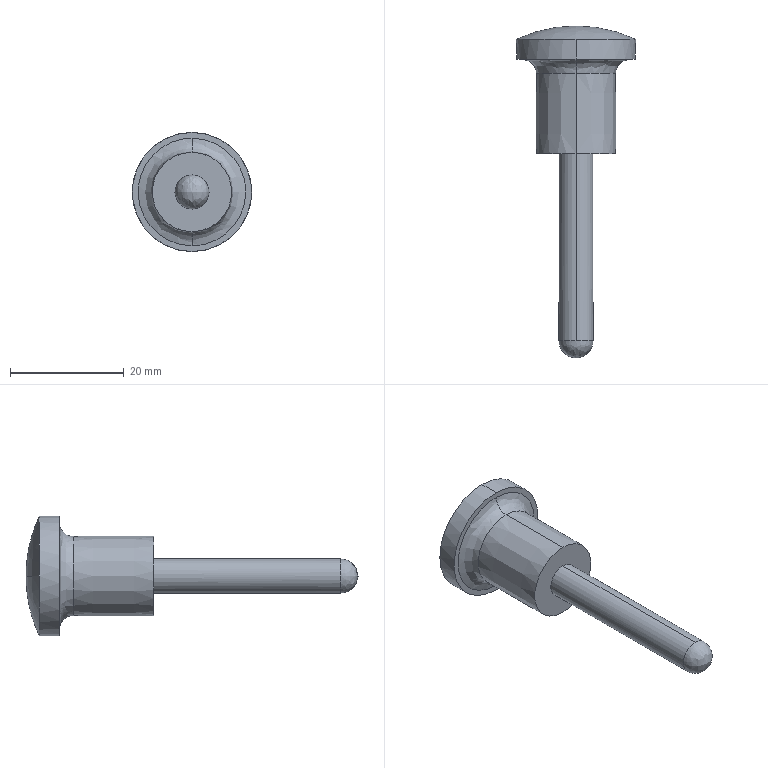Part | SolidWorks | features BaseBody 1 | 1 solid | 13 faces | box 21 x 58.38 x 21 mm | volume 5233 mm3 | spline 5 | cylinder 4 | cone 2 | plane 2 | commonest cylinder face diameters 6 x2 21 x2
STEP:
#1=CARTESIAN_POINT('',(0.,46.16,10.5));
#2=VERTEX_POINT('',#1);
#3=CARTESIAN_POINT('',(10.5,46.16,0.));
#4=VERTEX_POINT('',#3);
#5=CARTESIAN_POINT('',(0.,46.16,0.));
#6=DIRECTION('',(0.,1.,0.));
#7=DIRECTION('',(0.,0.,-1.));
#8=AXIS2_PLACEMENT_3D('',#5,#6,#7);
#9=CIRCLE('',#8,10.5);
#10=EDGE_CURVE('',#2,#4,#9,.T.);
#11=ORIENTED_EDGE('',*,*,#10,.T.);
#12=CARTESIAN_POINT('',(-10.5,46.16,0.));
#13=VERTEX_POINT('',#12);
#14=CARTESIAN_POINT('',(0.,23.772,0.));
#15=DIRECTION('',(0.,0.,1.));
#16=DIRECTION('',(1.,0.,0.));
#17=AXIS2_PLACEMENT_3D('',#14,#15,#16);
#18=CIRCLE('',#17,24.728);
#19=EDGE_CURVE('',#4,#13,#18,.T.);
#20=ORIENTED_EDGE('',*,*,#19,.T.);
#21=CARTESIAN_POINT('',(0.,46.16,0.));
#22=DIRECTION('',(0.,1.,0.));
#23=DIRECTION('',(0.,0.,-1.));
#24=AXIS2_PLACEMENT_3D('',#21,#22,#23);
#25=CIRCLE('',#24,10.5);
#26=EDGE_CURVE('',#13,#2,#25,.T.);
#27=ORIENTED_EDGE('',*,*,#26,.T.);
#28=EDGE_LOOP('',(#11,#20,#27));
#29=FACE_OUTER_BOUND('',#28,.T.);
#30=CARTESIAN_POINT('',(10.618,46.104,0.));
#31=CARTESIAN_POINT('',(10.618,46.104,3.311));
#32=CARTESIAN_POINT('',(10.618,45.38,6.542));
#33=CARTESIAN_POINT('',(10.618,43.966,9.536));
#34=CARTESIAN_POINT('',(3.784,49.354,0.));
#35=CARTESIAN_POINT('',(3.784,49.354,3.793));
#36=CARTESIAN_POINT('',(3.784,48.524,7.494));
#37=CARTESIAN_POINT('',(3.784,46.904,10.923));
#38=CARTESIAN_POINT('',(-3.784,49.354,0.));
#39=CARTESIAN_POINT('',(-3.784,49.354,3.793));
#40=CARTESIAN_POINT('',(-3.784,48.524,7.494));
#41=CARTESIAN_POINT('',(-3.784,46.904,10.923));
#42=CARTESIAN_POINT('',(-10.618,46.104,0.));
#43=CARTESIAN_POINT('',(-10.618,46.104,3.311));
#44=CARTESIAN_POINT('',(-10.618,45.38,6.542));
#45=CARTESIAN_POINT('',(-10.618,43.966,9.536));
#46=(BOUNDED_SURFACE()B_SPLINE_SURFACE(3,3,((#30,#31,#32,#33),(#34,#35,#36,#37),(#38,#39,#40,#41),(#42,#43,#44,#45)),.UNSPECIFIED.,.F.,.F.,.F.)B_SPLINE_SURFACE_WITH_KNOTS((4,4),(4,4),(0.,1.),(0.,1.),.UNSPECIFIED.)GEOMETRIC_REPRESENTATION_ITEM()RATIONAL_B_SPLINE_SURFACE(((1.,0.9838,0.9838,1.),(0.9354,0.9203,0.9203,0.9354),(0.9354,0.9203,0.9203,0.9354),(1.,0.9838,0.9838,1.)))REPRESENTATION_ITEM('')SURFACE());
#47=ADVANCED_FACE('',(#29),#46,.T.);
#48=CARTESIAN_POINT('',(0.,40.146,-6.975));
#49=VERTEX_POINT('',#48);
#50=CARTESIAN_POINT('',(0.,40.146,6.975));
#51=VERTEX_POINT('',#50);
#52=CARTESIAN_POINT('',(0.,40.146,0.));
#53=DIRECTION('',(0.,-1.,0.));
#54=DIRECTION('',(0.,0.,1.));
#55=AXIS2_PLACEMENT_3D('',#52,#53,#54);
#56=CIRCLE('',#55,6.975);
#57=EDGE_CURVE('',#49,#51,#56,.T.);
#58=ORIENTED_EDGE('',*,*,#57,.F.);
#59=CARTESIAN_POINT('',(0.,42.65,-9.475));
#60=VERTEX_POINT('',#59);
#61=CARTESIAN_POINT('',(0.,40.15,-9.475));
#62=DIRECTION('',(-1.,0.,0.));
#63=DIRECTION('',(0.,0.,-1.));
#64=AXIS2_PLACEMENT_3D('',#61,#62,#63);
#65=CIRCLE('',#64,2.5);
#66=EDGE_CURVE('',#49,#60,#65,.T.);
#67=ORIENTED_EDGE('',*,*,#66,.T.);
#68=CARTESIAN_POINT('',(9.475,42.65,0.));
#69=VERTEX_POINT('',#68);
#70=CARTESIAN_POINT('',(9.475,42.65,0.));
#71=CARTESIAN_POINT('',(9.475,42.65,-0.2897));
#72=CARTESIAN_POINT('',(9.456,42.65,-0.7225));
#73=CARTESIAN_POINT('',(9.398,42.65,-1.224));
#74=CARTESIAN_POINT('',(9.36,42.65,-1.475));
#75=CARTESIAN_POINT('',(9.342,42.65,-1.582));
#76=CARTESIAN_POINT('',(9.33,42.65,-1.653));
#77=CARTESIAN_POINT('',(9.324,42.65,-1.686));
#78=CARTESIAN_POINT('',(9.261,42.65,-2.026));
#79=CARTESIAN_POINT('',(9.156,42.65,-2.473));
#80=CARTESIAN_POINT('',(8.996,42.65,-2.984));
#81=CARTESIAN_POINT('',(8.906,42.65,-3.237));
#82=CARTESIAN_POINT('',(8.865,42.65,-3.345));
#83=CARTESIAN_POINT('',(8.838,42.65,-3.416));
#84=CARTESIAN_POINT('',(8.825,42.65,-3.451));
#85=CARTESIAN_POINT('',(8.692,42.65,-3.785));
#86=CARTESIAN_POINT('',(8.494,42.65,-4.221));
#87=CARTESIAN_POINT('',(8.225,42.65,-4.709));
#88=CARTESIAN_POINT('',(8.102,42.65,-4.915));
#89=CARTESIAN_POINT('',(8.018,42.65,-5.05));
#90=CARTESIAN_POINT('',(7.976,42.65,-5.117));
#91=CARTESIAN_POINT('',(7.573,42.65,-5.732));
#92=CARTESIAN_POINT('',(7.162,42.65,-6.238));
#93=CARTESIAN_POINT('',(6.469,42.65,-6.931));
#94=CARTESIAN_POINT('',(6.106,42.65,-7.258));
#95=CARTESIAN_POINT('',(5.655,42.65,-7.606));
#96=CARTESIAN_POINT('',(5.456,42.65,-7.748));
#97=CARTESIAN_POINT('',(5.321,42.65,-7.84));
#98=CARTESIAN_POINT('',(5.252,42.65,-7.887));
#99=CARTESIAN_POINT('',(4.917,42.65,-8.106));
#100=CARTESIAN_POINT('',(4.504,42.65,-8.347));
#101=CARTESIAN_POINT('',(4.003,42.65,-8.591));
#102=CARTESIAN_POINT('',(3.747,42.65,-8.704));
#103=CARTESIAN_POINT('',(3.636,42.65,-8.75));
#104=CARTESIAN_POINT('',(3.562,42.65,-8.78));
#105=CARTESIAN_POINT('',(3.524,42.65,-8.796));
#106=CARTESIAN_POINT('',(3.202,42.65,-8.923));
#107=CARTESIAN_POINT('',(2.768,42.65,-9.071));
#108=CARTESIAN_POINT('',(2.25,42.65,-9.207));
#109=CARTESIAN_POINT('',(1.988,42.65,-9.265));
#110=CARTESIAN_POINT('',(1.875,42.65,-9.288));
#111=CARTESIAN_POINT('',(1.8,42.65,-9.303));
#112=CARTESIAN_POINT('',(1.76,42.65,-9.311));
#113=CARTESIAN_POINT('',(1.154,42.65,-9.423));
#114=CARTESIAN_POINT('',(0.5797,42.65,-9.475));
#115=CARTESIAN_POINT('',(0.,42.65,-9.475));
#116=B_SPLINE_CURVE_WITH_KNOTS('',3,(#70,#71,#72,#73,#74,#75,#76,#77,#78,#79,#80,#81,#82,#83,#84,#85,#86,#87,#88,#89,#90,#91,#92,#93,#94,#95,#96,#97,#98,#99,#100,#101,#102,#103,#104,#105,#106,#107,#108,#109,#110,#111,#112,#113,#114,#115),.UNSPECIFIED.,.F.,.F.,(4,1,1,1,2,2,1,1,1,2,2,1,1,2,2,2,1,1,2,2,1,1,1,2,2,1,1,1,2,2,4),(0.,0.0625,0.09375,0.1094,0.1172,0.125,0.1875,0.2187,0.2344,0.2422,0.25,0.3125,0.3437,0.3594,0.375,0.5,0.5625,0.5938,0.6094,0.625,0.6875,0.7188,0.7344,0.7422,0.75,0.8125,0.8438,0.8594,0.8672,0.875,1.),.UNSPECIFIED.);
#117=EDGE_CURVE('',#69,#60,#116,.T.);
#118=ORIENTED_EDGE('',*,*,#117,.F.);
#119=CARTESIAN_POINT('',(0.,42.65,9.475));
#120=VERTEX_POINT('',#119);
#121=CARTESIAN_POINT('',(0.,42.65,9.475));
#122=CARTESIAN_POINT('',(0.2897,42.65,9.475));
#123=CARTESIAN_POINT('',(0.7225,42.65,9.456));
#124=CARTESIAN_POINT('',(1.224,42.65,9.398));
#125=CARTESIAN_POINT('',(1.475,42.65,9.36));
#126=CARTESIAN_POINT('',(1.582,42.65,9.342));
#127=CARTESIAN_POINT('',(1.653,42.65,9.33));
#128=CARTESIAN_POINT('',(1.686,42.65,9.324));
#129=CARTESIAN_POINT('',(2.026,42.65,9.261));
#130=CARTESIAN_POINT('',(2.473,42.65,9.156));
#131=CARTESIAN_POINT('',(2.984,42.65,8.996));
#132=CARTESIAN_POINT('',(3.237,42.65,8.906));
#133=CARTESIAN_POINT('',(3.345,42.65,8.865));
#134=CARTESIAN_POINT('',(3.416,42.65,8.838));
#135=CARTESIAN_POINT('',(3.451,42.65,8.825));
#136=CARTESIAN_POINT('',(3.785,42.65,8.692));
#137=CARTESIAN_POINT('',(4.221,42.65,8.494));
#138=CARTESIAN_POINT('',(4.709,42.65,8.225));
#139=CARTESIAN_POINT('',(4.915,42.65,8.102));
#140=CARTESIAN_POINT('',(5.05,42.65,8.018));
#141=CARTESIAN_POINT('',(5.117,42.65,7.976));
#142=CARTESIAN_POINT('',(5.732,42.65,7.573));
#143=CARTESIAN_POINT('',(6.238,42.65,7.162));
#144=CARTESIAN_POINT('',(6.931,42.65,6.469));
#145=CARTESIAN_POINT('',(7.258,42.65,6.106));
#146=CARTESIAN_POINT('',(7.606,42.65,5.655));
#147=CARTESIAN_POINT('',(7.748,42.65,5.456));
#148=CARTESIAN_POINT('',(7.84,42.65,5.321));
#149=CARTESIAN_POINT('',(7.887,42.65,5.252));
#150=CARTESIAN_POINT('',(8.106,42.65,4.917));
#151=CARTESIAN_POINT('',(8.347,42.65,4.504));
#152=CARTESIAN_POINT('',(8.591,42.65,4.003));
#153=CARTESIAN_POINT('',(8.704,42.65,3.747));
#154=CARTESIAN_POINT('',(8.75,42.65,3.636));
#155=CARTESIAN_POINT('',(8.78,42.65,3.562));
#156=CARTESIAN_POINT('',(8.796,42.65,3.524));
#157=CARTESIAN_POINT('',(8.923,42.65,3.202));
#158=CARTESIAN_POINT('',(9.071,42.65,2.768));
#159=CARTESIAN_POINT('',(9.207,42.65,2.25));
#160=CARTESIAN_POINT('',(9.265,42.65,1.988));
#161=CARTESIAN_POINT('',(9.288,42.65,1.875));
#162=CARTESIAN_POINT('',(9.303,42.65,1.8));
#163=CARTESIAN_POINT('',(9.311,42.65,1.76));
#164=CARTESIAN_POINT('',(9.423,42.65,1.154));
#165=CARTESIAN_POINT('',(9.475,42.65,0.5797));
#166=CARTESIAN_POINT('',(9.475,42.65,0.));
#167=B_SPLINE_CURVE_WITH_KNOTS('',3,(#121,#122,#123,#124,#125,#126,#127,#128,#129,#130,#131,#132,#133,#134,#135,#136,#137,#138,#139,#140,#141,#142,#143,#144,#145,#146,#147,#148,#149,#150,#151,#152,#153,#154,#155,#156,#157,#158,#159,#160,#161,#162,#163,#164,#165,#166),.UNSPECIFIED.,.F.,.F.,(4,1,1,1,2,2,1,1,1,2,2,1,1,2,2,2,1,1,2,2,1,1,1,2,2,1,1,1,2,2,4),(0.,0.0625,0.09375,0.1094,0.1172,0.125,0.1875,0.2188,0.2344,0.2422,0.25,0.3125,0.3438,0.3594,0.375,0.5,0.5625,0.5938,0.6094,0.625,0.6875,0.7188,0.7344,0.7422,0.75,0.8125,0.8438,0.8594,0.8672,0.875,1.),.UNSPECIFIED.);
#168=EDGE_CURVE('',#120,#69,#167,.T.);
#169=ORIENTED_EDGE('',*,*,#168,.F.);
#170=CARTESIAN_POINT('',(0.,40.15,9.475));
#171=DIRECTION('',(1.,0.,0.));
#172=DIRECTION('',(0.,0.,1.));
#173=AXIS2_PLACEMENT_3D('',#170,#171,#172);
#174=CIRCLE('',#173,2.5);
#175=EDGE_CURVE('',#51,#120,#174,.T.);
#176=ORIENTED_EDGE('',*,*,#175,.F.);
#177=EDGE_LOOP('',(#58,#67,#118,#169,#176));
#178=FACE_OUTER_BOUND('',#177,.T.);
#179=CARTESIAN_POINT('',(0.,40.146,6.975));
#180=CARTESIAN_POINT('',(13.951,40.146,6.975));
#181=CARTESIAN_POINT('',(13.951,40.146,-6.975));
#182=CARTESIAN_POINT('',(0.,40.146,-6.975));
#183=CARTESIAN_POINT('',(0.,41.612,6.973));
#184=CARTESIAN_POINT('',(13.946,41.612,6.973));
#185=CARTESIAN_POINT('',(13.946,41.612,-6.973));
#186=CARTESIAN_POINT('',(0.,41.612,-6.973));
#187=CARTESIAN_POINT('',(0.,42.65,8.009));
#188=CARTESIAN_POINT('',(16.018,42.65,8.009));
#189=CARTESIAN_POINT('',(16.018,42.65,-8.009));
#190=CARTESIAN_POINT('',(0.,42.65,-8.009));
#191=CARTESIAN_POINT('',(0.,42.65,9.475));
#192=CARTESIAN_POINT('',(18.951,42.65,9.475));
#193=CARTESIAN_POINT('',(18.951,42.65,-9.475));
#194=CARTESIAN_POINT('',(0.,42.65,-9.475));
#195=(BOUNDED_SURFACE()B_SPLINE_SURFACE(3,3,((#179,#180,#181,#182),(#183,#184,#185,#186),(#187,#188,#189,#190),(#191,#192,#193,#194)),.UNSPECIFIED.,.F.,.F.,.F.)B_SPLINE_SURFACE_WITH_KNOTS((4,4),(4,4),(0.,1.),(0.,1.),.UNSPECIFIED.)GEOMETRIC_REPRESENTATION_ITEM()RATIONAL_B_SPLINE_SURFACE(((1.,0.3333,0.3333,1.),(0.8043,0.2681,0.2681,0.8043),(0.8043,0.2681,0.2681,0.8043),(1.,0.3333,0.3333,1.)))REPRESENTATION_ITEM('')SURFACE());
#196=ADVANCED_FACE('',(#178),#195,.F.);
#197=ORIENTED_EDGE('',*,*,#10,.F.);
#198=CARTESIAN_POINT('',(0.,42.65,10.5));
#199=VERTEX_POINT('',#198);
#200=CARTESIAN_POINT('',(0.,44.405,10.5));
#201=DIRECTION('',(0.,-1.,0.));
#202=VECTOR('',#201,1000.);
#203=LINE('',#200,#202);
#204=EDGE_CURVE('',#2,#199,#203,.T.);
#205=ORIENTED_EDGE('',*,*,#204,.T.);
#206=CARTESIAN_POINT('',(0.,42.65,-10.5));
#207=VERTEX_POINT('',#206);
#208=CARTESIAN_POINT('',(0.,42.65,0.));
#209=DIRECTION('',(0.,1.,0.));
#210=DIRECTION('',(0.,0.,-1.));
#211=AXIS2_PLACEMENT_3D('',#208,#209,#210);
#212=CIRCLE('',#211,10.5);
#213=EDGE_CURVE('',#199,#207,#212,.T.);
#214=ORIENTED_EDGE('',*,*,#213,.T.);
#215=CARTESIAN_POINT('',(0.,46.16,-10.5));
#216=VERTEX_POINT('',#215);
#217=CARTESIAN_POINT('',(0.,44.405,-10.5));
#218=DIRECTION('',(0.,-1.,0.));
#219=VECTOR('',#218,1000.);
#220=LINE('',#217,#219);
#221=EDGE_CURVE('',#216,#207,#220,.T.);
#222=ORIENTED_EDGE('',*,*,#221,.F.);
#223=CARTESIAN_POINT('',(0.,46.16,0.));
#224=DIRECTION('',(0.,1.,0.));
#225=DIRECTION('',(0.,0.,-1.));
#226=AXIS2_PLACEMENT_3D('',#223,#224,#225);
#227=CIRCLE('',#226,10.5);
#228=EDGE_CURVE('',#4,#216,#227,.T.);
#229=ORIENTED_EDGE('',*,*,#228,.F.);
#230=EDGE_LOOP('',(#197,#205,#214,#222,#229));
#231=FACE_OUTER_BOUND('',#230,.T.);
#232=CARTESIAN_POINT('',(0.,44.405,0.));
#233=DIRECTION('',(0.,-1.,0.));
#234=DIRECTION('',(0.,0.,-1.));
#235=AXIS2_PLACEMENT_3D('',#232,#233,#234);
#236=CYLINDRICAL_SURFACE('',#235,10.5);
#237=ADVANCED_FACE('',(#231),#236,.T.);
#238=ORIENTED_EDGE('',*,*,#57,.T.);
#239=CARTESIAN_POINT('',(0.,26.,7.));
#240=VERTEX_POINT('',#239);
#241=CARTESIAN_POINT('',(0.,26.,7.));
#242=DIRECTION('',(0.,-1.,0.001745));
#243=VECTOR('',#242,1000.);
#244=LINE('',#241,#243);
#245=EDGE_CURVE('',#51,#240,#244,.T.);
#246=ORIENTED_EDGE('',*,*,#245,.T.);
#247=CARTESIAN_POINT('',(0.,26.,-7.));
#248=VERTEX_POINT('',#247);
#249=CARTESIAN_POINT('',(0.,26.,0.));
#250=DIRECTION('',(0.,1.,0.));
#251=DIRECTION('',(0.,0.,-1.));
#252=AXIS2_PLACEMENT_3D('',#249,#250,#251);
#253=CIRCLE('',#252,7.);
#254=EDGE_CURVE('',#240,#248,#253,.T.);
#255=ORIENTED_EDGE('',*,*,#254,.T.);
#256=CARTESIAN_POINT('',(0.,26.,-7.));
#257=DIRECTION('',(0.,-1.,-0.001745));
#258=VECTOR('',#257,1000.);
#259=LINE('',#256,#258);
#260=EDGE_CURVE('',#49,#248,#259,.T.);
#261=ORIENTED_EDGE('',*,*,#260,.F.);
#262=EDGE_LOOP('',(#238,#246,#255,#261));
#263=FACE_OUTER_BOUND('',#262,.T.);
#264=CARTESIAN_POINT('',(0.,26.,0.));
#265=DIRECTION('',(0.,-1.,0.));
#266=DIRECTION('',(0.,0.,-1.));
#267=AXIS2_PLACEMENT_3D('',#264,#265,#266);
#268=CONICAL_SURFACE('',#267,7.,0.001745);
#269=ADVANCED_FACE('',(#263),#268,.T.);
#270=CARTESIAN_POINT('',(0.,26.,3.));
#271=VERTEX_POINT('',#270);
#272=CARTESIAN_POINT('',(0.,26.,-3.));
#273=VERTEX_POINT('',#272);
#274=CARTESIAN_POINT('',(0.,26.,0.));
#275=DIRECTION('',(0.,1.,0.));
#276=DIRECTION('',(0.,0.,-1.));
#277=AXIS2_PLACEMENT_3D('',#274,#275,#276);
#278=CIRCLE('',#277,3.);
#279=EDGE_CURVE('',#271,#273,#278,.T.);
#280=ORIENTED_EDGE('',*,*,#279,.F.);
#281=CARTESIAN_POINT('',(0.,-7.,3.));
#282=VERTEX_POINT('',#281);
#283=CARTESIAN_POINT('',(0.,8.05,3.));
#284=DIRECTION('',(0.,-1.,0.));
#285=VECTOR('',#284,1000.);
#286=LINE('',#283,#285);
#287=EDGE_CURVE('',#271,#282,#286,.T.);
#288=ORIENTED_EDGE('',*,*,#287,.T.);
#289=CARTESIAN_POINT('',(3.,-7.,0.));
#290=VERTEX_POINT('',#289);
#291=CARTESIAN_POINT('',(0.,-7.,0.));
#292=DIRECTION('',(0.,1.,0.));
#293=DIRECTION('',(0.,0.,-1.));
#294=AXIS2_PLACEMENT_3D('',#291,#292,#293);
#295=CIRCLE('',#294,3.);
#296=EDGE_CURVE('',#282,#290,#295,.T.);
#297=ORIENTED_EDGE('',*,*,#296,.T.);
#298=CARTESIAN_POINT('',(0.,-7.,-3.));
#299=VERTEX_POINT('',#298);
#300=CARTESIAN_POINT('',(0.,-7.,0.));
#301=DIRECTION('',(0.,1.,0.));
#302=DIRECTION('',(0.,0.,-1.));
#303=AXIS2_PLACEMENT_3D('',#300,#301,#302);
#304=CIRCLE('',#303,3.);
#305=EDGE_CURVE('',#290,#299,#304,.T.);
#306=ORIENTED_EDGE('',*,*,#305,.T.);
#307=CARTESIAN_POINT('',(0.,8.05,-3.));
#308=DIRECTION('',(0.,-1.,0.));
#309=VECTOR('',#308,1000.);
#310=LINE('',#307,#309);
#311=EDGE_CURVE('',#273,#299,#310,.T.);
#312=ORIENTED_EDGE('',*,*,#311,.F.);
#313=EDGE_LOOP('',(#280,#288,#297,#306,#312));
#314=FACE_OUTER_BOUND('',#313,.T.);
#315=CARTESIAN_POINT('',(0.,8.05,0.));
#316=DIRECTION('',(0.,-1.,0.));
#317=DIRECTION('',(0.,0.,-1.));
#318=AXIS2_PLACEMENT_3D('',#315,#316,#317);
#319=CYLINDRICAL_SURFACE('',#318,3.);
#320=ADVANCED_FACE('',(#314),#319,.T.);
#321=ORIENTED_EDGE('',*,*,#19,.F.);
#322=ORIENTED_EDGE('',*,*,#228,.T.);
#323=CARTESIAN_POINT('',(0.,46.16,0.));
#324=DIRECTION('',(0.,1.,0.));
#325=DIRECTION('',(0.,0.,-1.));
#326=AXIS2_PLACEMENT_3D('',#323,#324,#325);
#327=CIRCLE('',#326,10.5);
#328=EDGE_CURVE('',#216,#13,#327,.T.);
#329=ORIENTED_EDGE('',*,*,#328,.T.);
#330=EDGE_LOOP('',(#321,#322,#329));
#331=FACE_OUTER_BOUND('',#330,.T.);
#332=CARTESIAN_POINT('',(10.618,43.966,-9.536));
#333=CARTESIAN_POINT('',(10.618,45.38,-6.542));
#334=CARTESIAN_POINT('',(10.618,46.104,-3.311));
#335=CARTESIAN_POINT('',(10.618,46.104,0.));
#336=CARTESIAN_POINT('',(3.784,46.904,-10.923));
#337=CARTESIAN_POINT('',(3.784,48.524,-7.494));
#338=CARTESIAN_POINT('',(3.784,49.354,-3.793));
#339=CARTESIAN_POINT('',(3.784,49.354,0.));
#340=CARTESIAN_POINT('',(-3.784,46.904,-10.923));
#341=CARTESIAN_POINT('',(-3.784,48.524,-7.494));
#342=CARTESIAN_POINT('',(-3.784,49.354,-3.793));
#343=CARTESIAN_POINT('',(-3.784,49.354,0.));
#344=CARTESIAN_POINT('',(-10.618,43.966,-9.536));
#345=CARTESIAN_POINT('',(-10.618,45.38,-6.542));
#346=CARTESIAN_POINT('',(-10.618,46.104,-3.311));
#347=CARTESIAN_POINT('',(-10.618,46.104,0.));
#348=(BOUNDED_SURFACE()B_SPLINE_SURFACE(3,3,((#332,#333,#334,#335),(#336,#337,#338,#339),(#340,#341,#342,#343),(#344,#345,#346,#347)),.UNSPECIFIED.,.F.,.F.,.F.)B_SPLINE_SURFACE_WITH_KNOTS((4,4),(4,4),(0.,1.),(0.,1.),.UNSPECIFIED.)GEOMETRIC_REPRESENTATION_ITEM()RATIONAL_B_SPLINE_SURFACE(((1.,0.9838,0.9838,1.),(0.9354,0.9203,0.9203,0.9354),(0.9354,0.9203,0.9203,0.9354),(1.,0.9838,0.9838,1.)))REPRESENTATION_ITEM('')SURFACE());
#349=ADVANCED_FACE('',(#331),#348,.T.);
#350=ORIENTED_EDGE('',*,*,#204,.F.);
#351=ORIENTED_EDGE('',*,*,#26,.F.);
#352=ORIENTED_EDGE('',*,*,#328,.F.);
#353=ORIENTED_EDGE('',*,*,#221,.T.);
#354=CARTESIAN_POINT('',(0.,42.65,0.));
#355=DIRECTION('',(0.,1.,0.));
#356=DIRECTION('',(0.,0.,-1.));
#357=AXIS2_PLACEMENT_3D('',#354,#355,#356);
#358=CIRCLE('',#357,10.5);
#359=EDGE_CURVE('',#207,#199,#358,.T.);
#360=ORIENTED_EDGE('',*,*,#359,.T.);
#361=EDGE_LOOP('',(#350,#351,#352,#353,#360));
#362=FACE_OUTER_BOUND('',#361,.T.);
#363=CARTESIAN_POINT('',(0.,44.405,0.));
#364=DIRECTION('',(0.,-1.,0.));
#365=DIRECTION('',(0.,0.,-1.));
#366=AXIS2_PLACEMENT_3D('',#363,#364,#365);
#367=CYLINDRICAL_SURFACE('',#366,10.5);
#368=ADVANCED_FACE('',(#362),#367,.T.);
#369=CARTESIAN_POINT('',(0.,42.65,-9.475));
#370=CARTESIAN_POINT('',(-0.2897,42.65,-9.475));
#371=CARTESIAN_POINT('',(-0.7225,42.65,-9.456));
#372=CARTESIAN_POINT('',(-1.224,42.65,-9.398));
#373=CARTESIAN_POINT('',(-1.475,42.65,-9.36));
#374=CARTESIAN_POINT('',(-1.582,42.65,-9.342));
#375=CARTESIAN_POINT('',(-1.653,42.65,-9.33));
#376=CARTESIAN_POINT('',(-1.686,42.65,-9.324));
#377=CARTESIAN_POINT('',(-2.026,42.65,-9.261));
#378=CARTESIAN_POINT('',(-2.473,42.65,-9.156));
#379=CARTESIAN_POINT('',(-2.984,42.65,-8.996));
#380=CARTESIAN_POINT('',(-3.237,42.65,-8.906));
#381=CARTESIAN_POINT('',(-3.345,42.65,-8.865));
#382=CARTESIAN_POINT('',(-3.416,42.65,-8.838));
#383=CARTESIAN_POINT('',(-3.451,42.65,-8.825));
#384=CARTESIAN_POINT('',(-3.785,42.65,-8.692));
#385=CARTESIAN_POINT('',(-4.221,42.65,-8.494));
#386=CARTESIAN_POINT('',(-4.709,42.65,-8.225));
#387=CARTESIAN_POINT('',(-4.915,42.65,-8.102));
#388=CARTESIAN_POINT('',(-5.05,42.65,-8.018));
#389=CARTESIAN_POINT('',(-5.117,42.65,-7.976));
#390=CARTESIAN_POINT('',(-5.732,42.65,-7.573));
#391=CARTESIAN_POINT('',(-6.238,42.65,-7.162));
#392=CARTESIAN_POINT('',(-6.931,42.65,-6.469));
#393=CARTESIAN_POINT('',(-7.258,42.65,-6.106));
#394=CARTESIAN_POINT('',(-7.606,42.65,-5.655));
#395=CARTESIAN_POINT('',(-7.748,42.65,-5.456));
#396=CARTESIAN_POINT('',(-7.84,42.65,-5.321));
#397=CARTESIAN_POINT('',(-7.887,42.65,-5.252));
#398=CARTESIAN_POINT('',(-8.106,42.65,-4.917));
#399=CARTESIAN_POINT('',(-8.347,42.65,-4.504));
#400=CARTESIAN_POINT('',(-8.591,42.65,-4.003));
#401=CARTESIAN_POINT('',(-8.704,42.65,-3.747));
#402=CARTESIAN_POINT('',(-8.75,42.65,-3.636));
#403=CARTESIAN_POINT('',(-8.78,42.65,-3.562));
#404=CARTESIAN_POINT('',(-8.796,42.65,-3.524));
#405=CARTESIAN_POINT('',(-8.923,42.65,-3.202));
#406=CARTESIAN_POINT('',(-9.071,42.65,-2.768));
#407=CARTESIAN_POINT('',(-9.207,42.65,-2.25));
#408=CARTESIAN_POINT('',(-9.265,42.65,-1.988));
#409=CARTESIAN_POINT('',(-9.288,42.65,-1.875));
#410=CARTESIAN_POINT('',(-9.303,42.65,-1.8));
#411=CARTESIAN_POINT('',(-9.311,42.65,-1.76));
#412=CARTESIAN_POINT('',(-9.423,42.65,-1.155));
#413=CARTESIAN_POINT('',(-9.475,42.65,-0.5792));
#414=CARTESIAN_POINT('',(-9.475,42.65,0.2896));
#415=CARTESIAN_POINT('',(-9.456,42.65,0.7223));
#416=CARTESIAN_POINT('',(-9.398,42.65,1.224));
#417=CARTESIAN_POINT('',(-9.36,42.65,1.474));
#418=CARTESIAN_POINT('',(-9.342,42.65,1.582));
#419=CARTESIAN_POINT('',(-9.33,42.65,1.653));
#420=CARTESIAN_POINT('',(-9.324,42.65,1.686));
#421=CARTESIAN_POINT('',(-9.261,42.65,2.026));
#422=CARTESIAN_POINT('',(-9.156,42.65,2.473));
#423=CARTESIAN_POINT('',(-8.996,42.65,2.984));
#424=CARTESIAN_POINT('',(-8.906,42.65,3.237));
#425=CARTESIAN_POINT('',(-8.865,42.65,3.345));
#426=CARTESIAN_POINT('',(-8.838,42.65,3.416));
#427=CARTESIAN_POINT('',(-8.825,42.65,3.451));
#428=CARTESIAN_POINT('',(-8.692,42.65,3.785));
#429=CARTESIAN_POINT('',(-8.494,42.65,4.221));
#430=CARTESIAN_POINT('',(-8.225,42.65,4.709));
#431=CARTESIAN_POINT('',(-8.102,42.65,4.915));
#432=CARTESIAN_POINT('',(-8.018,42.65,5.05));
#433=CARTESIAN_POINT('',(-7.976,42.65,5.117));
#434=CARTESIAN_POINT('',(-7.573,42.65,5.732));
#435=CARTESIAN_POINT('',(-7.162,42.65,6.238));
#436=CARTESIAN_POINT('',(-6.469,42.65,6.931));
#437=CARTESIAN_POINT('',(-6.106,42.65,7.258));
#438=CARTESIAN_POINT('',(-5.655,42.65,7.606));
#439=CARTESIAN_POINT('',(-5.456,42.65,7.748));
#440=CARTESIAN_POINT('',(-5.321,42.65,7.84));
#441=CARTESIAN_POINT('',(-5.252,42.65,7.887));
#442=CARTESIAN_POINT('',(-4.917,42.65,8.106));
#443=CARTESIAN_POINT('',(-4.504,42.65,8.347));
#444=CARTESIAN_POINT('',(-4.003,42.65,8.591));
#445=CARTESIAN_POINT('',(-3.747,42.65,8.704));
#446=CARTESIAN_POINT('',(-3.636,42.65,8.75));
#447=CARTESIAN_POINT('',(-3.562,42.65,8.78));
#448=CARTESIAN_POINT('',(-3.524,42.65,8.796));
#449=CARTESIAN_POINT('',(-3.202,42.65,8.923));
#450=CARTESIAN_POINT('',(-2.768,42.65,9.071));
#451=CARTESIAN_POINT('',(-2.25,42.65,9.207));
#452=CARTESIAN_POINT('',(-1.988,42.65,9.265));
#453=CARTESIAN_POINT('',(-1.875,42.65,9.288));
#454=CARTESIAN_POINT('',(-1.8,42.65,9.303));
#455=CARTESIAN_POINT('',(-1.76,42.65,9.311));
#456=CARTESIAN_POINT('',(-1.154,42.65,9.423));
#457=CARTESIAN_POINT('',(-0.5797,42.65,9.475));
#458=CARTESIAN_POINT('',(0.,42.65,9.475));
#459=B_SPLINE_CURVE_WITH_KNOTS('',3,(#369,#370,#371,#372,#373,#374,#375,#376,#377,#378,#379,#380,#381,#382,#383,#384,#385,#386,#387,#388,#389,#390,#391,#392,#393,#394,#395,#396,#397,#398,#399,#400,#401,#402,#403,#404,#405,#406,#407,#408,#409,#410,#411,#412,#413,#414,#415,#416,#417,#418,#419,#420,#421,#422,#423,#424,#425,#426,#427,#428,#429,#430,#431,#432,#433,#434,#435,#436,#437,#438,#439,#440,#441,#442,#443,#444,#445,#446,#447,#448,#449,#450,#451,#452,#453,#454,#455,#456,#457,#458),.UNSPECIFIED.,.F.,.F.,(4,1,1,1,2,2,1,1,1,2,2,1,1,2,2,2,1,1,2,2,1,1,1,2,2,1,1,1,2,2,2,1,1,1,2,2,1,1,1,2,2,1,1,2,2,2,1,1,2,2,1,1,1,2,2,1,1,1,2,2,4),(0.,0.03125,0.04687,0.05469,0.05859,0.0625,0.09375,0.1094,0.1172,0.1211,0.125,0.1562,0.1719,0.1797,0.1875,0.25,0.2812,0.2969,0.3047,0.3125,0.3437,0.3594,0.3672,0.3711,0.375,0.4062,0.4219,0.4297,0.4336,0.4375,0.5,0.5312,0.5469,0.5547,0.5586,0.5625,0.5937,0.6094,0.6172,0.6211,0.625,0.6563,0.6719,0.6797,0.6875,0.75,0.7812,0.7969,0.8047,0.8125,0.8437,0.8594,0.8672,0.8711,0.875,0.9062,0.9219,0.9297,0.9336,0.9375,1.),.UNSPECIFIED.);
#460=EDGE_CURVE('',#60,#120,#459,.T.);
#461=ORIENTED_EDGE('',*,*,#460,.T.);
#462=ORIENTED_EDGE('',*,*,#168,.T.);
#463=ORIENTED_EDGE('',*,*,#117,.T.);
#464=EDGE_LOOP('',(#461,#462,#463));
#465=FACE_BOUND('',#464,.T.);
#466=ORIENTED_EDGE('',*,*,#359,.F.);
#467=ORIENTED_EDGE('',*,*,#213,.F.);
#468=EDGE_LOOP('',(#466,#467));
#469=FACE_OUTER_BOUND('',#468,.T.);
#470=CARTESIAN_POINT('',(9.988,42.65,0.));
#471=DIRECTION('',(0.,-1.,0.));
#472=DIRECTION('',(0.,0.,-1.));
#473=AXIS2_PLACEMENT_3D('',#470,#471,#472);
#474=PLANE('',#473);
#475=ADVANCED_FACE('',(#465,#469),#474,.T.);
#476=ORIENTED_EDGE('',*,*,#66,.F.);
#477=CARTESIAN_POINT('',(0.,40.146,0.));
#478=DIRECTION('',(0.,-1.,0.));
#479=DIRECTION('',(0.,0.,1.));
#480=AXIS2_PLACEMENT_3D('',#477,#478,#479);
#481=CIRCLE('',#480,6.975);
#482=EDGE_CURVE('',#51,#49,#481,.T.);
#483=ORIENTED_EDGE('',*,*,#482,.F.);
#484=ORIENTED_EDGE('',*,*,#175,.T.);
#485=ORIENTED_EDGE('',*,*,#460,.F.);
#486=EDGE_LOOP('',(#476,#483,#484,#485));
#487=FACE_OUTER_BOUND('',#486,.T.);
#488=CARTESIAN_POINT('',(0.,40.146,-6.975));
#489=CARTESIAN_POINT('',(-13.951,40.146,-6.975));
#490=CARTESIAN_POINT('',(-13.951,40.146,6.975));
#491=CARTESIAN_POINT('',(0.,40.146,6.975));
#492=CARTESIAN_POINT('',(0.,41.612,-6.973));
#493=CARTESIAN_POINT('',(-13.946,41.612,-6.973));
#494=CARTESIAN_POINT('',(-13.946,41.612,6.973));
#495=CARTESIAN_POINT('',(0.,41.612,6.973));
#496=CARTESIAN_POINT('',(0.,42.65,-8.009));
#497=CARTESIAN_POINT('',(-16.018,42.65,-8.009));
#498=CARTESIAN_POINT('',(-16.018,42.65,8.009));
#499=CARTESIAN_POINT('',(0.,42.65,8.009));
#500=CARTESIAN_POINT('',(0.,42.65,-9.475));
#501=CARTESIAN_POINT('',(-18.951,42.65,-9.475));
#502=CARTESIAN_POINT('',(-18.951,42.65,9.475));
#503=CARTESIAN_POINT('',(0.,42.65,9.475));
#504=(BOUNDED_SURFACE()B_SPLINE_SURFACE(3,3,((#488,#489,#490,#491),(#492,#493,#494,#495),(#496,#497,#498,#499),(#500,#501,#502,#503)),.UNSPECIFIED.,.F.,.F.,.F.)B_SPLINE_SURFACE_WITH_KNOTS((4,4),(4,4),(0.,1.),(0.,1.),.UNSPECIFIED.)GEOMETRIC_REPRESENTATION_ITEM()RATIONAL_B_SPLINE_SURFACE(((1.,0.3333,0.3333,1.),(0.8043,0.2681,0.2681,0.8043),(0.8043,0.2681,0.2681,0.8043),(1.,0.3333,0.3333,1.)))REPRESENTATION_ITEM('')SURFACE());
#505=ADVANCED_FACE('',(#487),#504,.F.);
#506=ORIENTED_EDGE('',*,*,#245,.F.);
#507=ORIENTED_EDGE('',*,*,#482,.T.);
#508=ORIENTED_EDGE('',*,*,#260,.T.);
#509=CARTESIAN_POINT('',(0.,26.,0.));
#510=DIRECTION('',(0.,1.,0.));
#511=DIRECTION('',(0.,0.,-1.));
#512=AXIS2_PLACEMENT_3D('',#509,#510,#511);
#513=CIRCLE('',#512,7.);
#514=EDGE_CURVE('',#248,#240,#513,.T.);
#515=ORIENTED_EDGE('',*,*,#514,.T.);
#516=EDGE_LOOP('',(#506,#507,#508,#515));
#517=FACE_OUTER_BOUND('',#516,.T.);
#518=CARTESIAN_POINT('',(0.,26.,0.));
#519=DIRECTION('',(0.,-1.,0.));
#520=DIRECTION('',(0.,0.,-1.));
#521=AXIS2_PLACEMENT_3D('',#518,#519,#520);
#522=CONICAL_SURFACE('',#521,7.,0.001745);
#523=ADVANCED_FACE('',(#517),#522,.T.);
#524=CARTESIAN_POINT('',(0.,26.,0.));
#525=DIRECTION('',(0.,1.,0.));
#526=DIRECTION('',(0.,0.,-1.));
#527=AXIS2_PLACEMENT_3D('',#524,#525,#526);
#528=CIRCLE('',#527,3.);
#529=EDGE_CURVE('',#273,#271,#528,.T.);
#530=ORIENTED_EDGE('',*,*,#529,.T.);
#531=ORIENTED_EDGE('',*,*,#279,.T.);
#532=EDGE_LOOP('',(#530,#531));
#533=FACE_BOUND('',#532,.T.);
#534=ORIENTED_EDGE('',*,*,#514,.F.);
#535=ORIENTED_EDGE('',*,*,#254,.F.);
#536=EDGE_LOOP('',(#534,#535));
#537=FACE_OUTER_BOUND('',#536,.T.);
#538=CARTESIAN_POINT('',(5.,26.,0.));
#539=DIRECTION('',(0.,-1.,0.));
#540=DIRECTION('',(0.,0.,-1.));
#541=AXIS2_PLACEMENT_3D('',#538,#539,#540);
#542=PLANE('',#541);
#543=ADVANCED_FACE('',(#533,#537),#542,.T.);
#544=ORIENTED_EDGE('',*,*,#287,.F.);
#545=ORIENTED_EDGE('',*,*,#529,.F.);
#546=ORIENTED_EDGE('',*,*,#311,.T.);
#547=CARTESIAN_POINT('',(-3.,-7.,0.));
#548=VERTEX_POINT('',#547);
#549=CARTESIAN_POINT('',(0.,-7.,0.));
#550=DIRECTION('',(0.,1.,0.));
#551=DIRECTION('',(0.,0.,-1.));
#552=AXIS2_PLACEMENT_3D('',#549,#550,#551);
#553=CIRCLE('',#552,3.);
#554=EDGE_CURVE('',#299,#548,#553,.T.);
#555=ORIENTED_EDGE('',*,*,#554,.T.);
#556=CARTESIAN_POINT('',(0.,-7.,0.));
#557=DIRECTION('',(0.,1.,0.));
#558=DIRECTION('',(0.,0.,-1.));
#559=AXIS2_PLACEMENT_3D('',#556,#557,#558);
#560=CIRCLE('',#559,3.);
#561=EDGE_CURVE('',#548,#282,#560,.T.);
#562=ORIENTED_EDGE('',*,*,#561,.T.);
#563=EDGE_LOOP('',(#544,#545,#546,#555,#562));
#564=FACE_OUTER_BOUND('',#563,.T.);
#565=CARTESIAN_POINT('',(0.,8.05,0.));
#566=DIRECTION('',(0.,-1.,0.));
#567=DIRECTION('',(0.,0.,-1.));
#568=AXIS2_PLACEMENT_3D('',#565,#566,#567);
#569=CYLINDRICAL_SURFACE('',#568,3.);
#570=ADVANCED_FACE('',(#564),#569,.T.);
#571=ORIENTED_EDGE('',*,*,#561,.F.);
#572=ORIENTED_EDGE('',*,*,#554,.F.);
#573=ORIENTED_EDGE('',*,*,#305,.F.);
#574=ORIENTED_EDGE('',*,*,#296,.F.);
#575=EDGE_LOOP('',(#571,#572,#573,#574));
#576=FACE_OUTER_BOUND('',#575,.T.);
#577=CARTESIAN_POINT('',(3.,-7.,0.));
#578=CARTESIAN_POINT('',(3.,-7.,0.));
#579=CARTESIAN_POINT('',(3.,-7.,0.));
#580=CARTESIAN_POINT('',(3.,-7.,0.));
#581=CARTESIAN_POINT('',(3.,-7.,6.));
#582=CARTESIAN_POINT('',(3.,-19.,6.));
#583=CARTESIAN_POINT('',(3.,-19.,-6.));
#584=CARTESIAN_POINT('',(3.,-7.,-6.));
#585=CARTESIAN_POINT('',(-3.,-7.,6.));
#586=CARTESIAN_POINT('',(-3.,-19.,6.));
#587=CARTESIAN_POINT('',(-3.,-19.,-6.));
#588=CARTESIAN_POINT('',(-3.,-7.,-6.));
#589=CARTESIAN_POINT('',(-3.,-7.,0.));
#590=CARTESIAN_POINT('',(-3.,-7.,0.));
#591=CARTESIAN_POINT('',(-3.,-7.,0.));
#592=CARTESIAN_POINT('',(-3.,-7.,0.));
#593=(BOUNDED_SURFACE()B_SPLINE_SURFACE(3,3,((#577,#578,#579,#580),(#581,#582,#583,#584),(#585,#586,#587,#588),(#589,#590,#591,#592)),.UNSPECIFIED.,.F.,.F.,.F.)B_SPLINE_SURFACE_WITH_KNOTS((4,4),(4,4),(0.,1.),(0.,1.),.UNSPECIFIED.)GEOMETRIC_REPRESENTATION_ITEM()RATIONAL_B_SPLINE_SURFACE(((1.,0.3333,0.3333,1.),(0.3333,0.1111,0.1111,0.3333),(0.3333,0.1111,0.1111,0.3333),(1.,0.3333,0.3333,1.)))REPRESENTATION_ITEM('')SURFACE());
#594=ADVANCED_FACE('',(#576),#593,.T.);
#595=CLOSED_SHELL('',(#47,#196,#237,#269,#320,#349,#368,#475,#505,#523,#543,#570,#594));
#596=MANIFOLD_SOLID_BREP('',#595);
#597=CARTESIAN_POINT('',(0.,0.,0.));
#598=DIRECTION('',(0.,0.,1.));
#599=DIRECTION('',(1.,0.,0.));
#600=AXIS2_PLACEMENT_3D('',#597,#598,#599);
#601=(LENGTH_UNIT()NAMED_UNIT(*)SI_UNIT(.MILLI.,.METRE.));
#602=UNCERTAINTY_MEASURE_WITH_UNIT(LENGTH_MEASURE(0.00001),#601,'','');
#603=(NAMED_UNIT(*)PLANE_ANGLE_UNIT()SI_UNIT($,.RADIAN.));
#604=(NAMED_UNIT(*)SI_UNIT($,.STERADIAN.)SOLID_ANGLE_UNIT());
#605=(GEOMETRIC_REPRESENTATION_CONTEXT(3)GLOBAL_UNCERTAINTY_ASSIGNED_CONTEXT((#602))GLOBAL_UNIT_ASSIGNED_CONTEXT((#601,#603,#604))REPRESENTATION_CONTEXT('',''));
#606=ADVANCED_BREP_SHAPE_REPRESENTATION('',(#596,#600),#605);